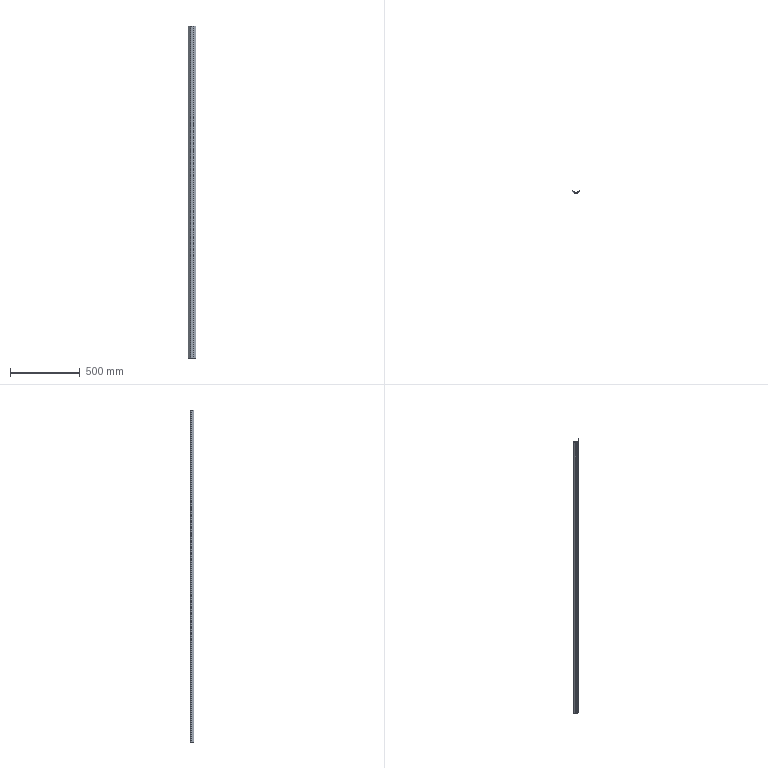Part | SolidWorks | features Extrusion 1 | 1 solid | 40 faces | box 56.572 x 22.358 x 2385 mm | volume 399812 mm3 | plane 37 | cylinder 3 | commonest cylinder face diameters 1 x2 0.5 x1
STEP:
#1=CARTESIAN_POINT('',(6.75,2.,-1192.5));
#2=VERTEX_POINT('',#1);
#3=CARTESIAN_POINT('',(6.75,5.,-1192.5));
#4=VERTEX_POINT('',#3);
#5=CARTESIAN_POINT('',(6.75,2.,-1192.5));
#6=DIRECTION('',(0.,1.,0.));
#7=VECTOR('',#6,1000.);
#8=LINE('',#5,#7);
#9=EDGE_CURVE('',#2,#4,#8,.T.);
#10=ORIENTED_EDGE('',*,*,#9,.T.);
#11=CARTESIAN_POINT('',(6.75,5.,1192.5));
#12=VERTEX_POINT('',#11);
#13=CARTESIAN_POINT('',(6.75,5.,1192.5));
#14=DIRECTION('',(0.,0.,-1.));
#15=VECTOR('',#14,1000.);
#16=LINE('',#13,#15);
#17=EDGE_CURVE('',#12,#4,#16,.T.);
#18=ORIENTED_EDGE('',*,*,#17,.F.);
#19=CARTESIAN_POINT('',(6.75,2.,1192.5));
#20=VERTEX_POINT('',#19);
#21=CARTESIAN_POINT('',(6.75,2.,1192.5));
#22=DIRECTION('',(0.,1.,0.));
#23=VECTOR('',#22,1000.);
#24=LINE('',#21,#23);
#25=EDGE_CURVE('',#20,#12,#24,.T.);
#26=ORIENTED_EDGE('',*,*,#25,.F.);
#27=CARTESIAN_POINT('',(6.75,2.,1192.5));
#28=DIRECTION('',(0.,0.,-1.));
#29=VECTOR('',#28,1000.);
#30=LINE('',#27,#29);
#31=EDGE_CURVE('',#20,#2,#30,.T.);
#32=ORIENTED_EDGE('',*,*,#31,.T.);
#33=EDGE_LOOP('',(#10,#18,#26,#32));
#34=FACE_OUTER_BOUND('',#33,.T.);
#35=CARTESIAN_POINT('',(6.75,2.,1192.5));
#36=DIRECTION('',(-1.,0.,0.));
#37=DIRECTION('',(0.,0.,1.));
#38=AXIS2_PLACEMENT_3D('',#35,#36,#37);
#39=PLANE('',#38);
#40=ADVANCED_FACE('',(#34),#39,.F.);
#41=CARTESIAN_POINT('',(5.25,5.,-1192.5));
#42=VERTEX_POINT('',#41);
#43=CARTESIAN_POINT('',(6.75,5.,-1192.5));
#44=DIRECTION('',(-1.,0.,0.));
#45=VECTOR('',#44,1000.);
#46=LINE('',#43,#45);
#47=EDGE_CURVE('',#4,#42,#46,.T.);
#48=ORIENTED_EDGE('',*,*,#47,.T.);
#49=CARTESIAN_POINT('',(5.25,5.,1192.5));
#50=VERTEX_POINT('',#49);
#51=CARTESIAN_POINT('',(5.25,5.,1192.5));
#52=DIRECTION('',(0.,0.,-1.));
#53=VECTOR('',#52,1000.);
#54=LINE('',#51,#53);
#55=EDGE_CURVE('',#50,#42,#54,.T.);
#56=ORIENTED_EDGE('',*,*,#55,.F.);
#57=CARTESIAN_POINT('',(6.75,5.,1192.5));
#58=DIRECTION('',(-1.,0.,0.));
#59=VECTOR('',#58,1000.);
#60=LINE('',#57,#59);
#61=EDGE_CURVE('',#12,#50,#60,.T.);
#62=ORIENTED_EDGE('',*,*,#61,.F.);
#63=ORIENTED_EDGE('',*,*,#17,.T.);
#64=EDGE_LOOP('',(#48,#56,#62,#63));
#65=FACE_OUTER_BOUND('',#64,.T.);
#66=CARTESIAN_POINT('',(6.75,5.,1192.5));
#67=DIRECTION('',(0.,-1.,0.));
#68=DIRECTION('',(1.,0.,0.));
#69=AXIS2_PLACEMENT_3D('',#66,#67,#68);
#70=PLANE('',#69);
#71=ADVANCED_FACE('',(#65),#70,.F.);
#72=CARTESIAN_POINT('',(5.25,2.,-1192.5));
#73=VERTEX_POINT('',#72);
#74=CARTESIAN_POINT('',(5.25,5.,-1192.5));
#75=DIRECTION('',(0.,-1.,0.));
#76=VECTOR('',#75,1000.);
#77=LINE('',#74,#76);
#78=EDGE_CURVE('',#42,#73,#77,.T.);
#79=ORIENTED_EDGE('',*,*,#78,.T.);
#80=CARTESIAN_POINT('',(5.25,2.,1192.5));
#81=VERTEX_POINT('',#80);
#82=CARTESIAN_POINT('',(5.25,2.,1192.5));
#83=DIRECTION('',(0.,0.,-1.));
#84=VECTOR('',#83,1000.);
#85=LINE('',#82,#84);
#86=EDGE_CURVE('',#81,#73,#85,.T.);
#87=ORIENTED_EDGE('',*,*,#86,.F.);
#88=CARTESIAN_POINT('',(5.25,5.,1192.5));
#89=DIRECTION('',(0.,-1.,0.));
#90=VECTOR('',#89,1000.);
#91=LINE('',#88,#90);
#92=EDGE_CURVE('',#50,#81,#91,.T.);
#93=ORIENTED_EDGE('',*,*,#92,.F.);
#94=ORIENTED_EDGE('',*,*,#55,.T.);
#95=EDGE_LOOP('',(#79,#87,#93,#94));
#96=FACE_OUTER_BOUND('',#95,.T.);
#97=CARTESIAN_POINT('',(5.25,5.,1192.5));
#98=DIRECTION('',(1.,0.,0.));
#99=DIRECTION('',(0.,0.,-1.));
#100=AXIS2_PLACEMENT_3D('',#97,#98,#99);
#101=PLANE('',#100);
#102=ADVANCED_FACE('',(#96),#101,.F.);
#103=CARTESIAN_POINT('',(0.25,2.,-1192.5));
#104=VERTEX_POINT('',#103);
#105=CARTESIAN_POINT('',(5.25,2.,-1192.5));
#106=DIRECTION('',(-1.,0.,0.));
#107=VECTOR('',#106,1000.);
#108=LINE('',#105,#107);
#109=EDGE_CURVE('',#73,#104,#108,.T.);
#110=ORIENTED_EDGE('',*,*,#109,.T.);
#111=CARTESIAN_POINT('',(0.25,2.,1192.5));
#112=VERTEX_POINT('',#111);
#113=CARTESIAN_POINT('',(0.25,2.,1192.5));
#114=DIRECTION('',(0.,0.,-1.));
#115=VECTOR('',#114,1000.);
#116=LINE('',#113,#115);
#117=EDGE_CURVE('',#112,#104,#116,.T.);
#118=ORIENTED_EDGE('',*,*,#117,.F.);
#119=CARTESIAN_POINT('',(5.25,2.,1192.5));
#120=DIRECTION('',(-1.,0.,0.));
#121=VECTOR('',#120,1000.);
#122=LINE('',#119,#121);
#123=EDGE_CURVE('',#81,#112,#122,.T.);
#124=ORIENTED_EDGE('',*,*,#123,.F.);
#125=ORIENTED_EDGE('',*,*,#86,.T.);
#126=EDGE_LOOP('',(#110,#118,#124,#125));
#127=FACE_OUTER_BOUND('',#126,.T.);
#128=CARTESIAN_POINT('',(5.25,2.,1192.5));
#129=DIRECTION('',(0.,-1.,0.));
#130=DIRECTION('',(0.,0.,-1.));
#131=AXIS2_PLACEMENT_3D('',#128,#129,#130);
#132=PLANE('',#131);
#133=ADVANCED_FACE('',(#127),#132,.F.);
#134=CARTESIAN_POINT('',(-0.25,2.,-1192.5));
#135=VERTEX_POINT('',#134);
#136=CARTESIAN_POINT('',(0.,2.,-1192.5));
#137=DIRECTION('',(0.,0.,-1.));
#138=DIRECTION('',(1.,0.,0.));
#139=AXIS2_PLACEMENT_3D('',#136,#137,#138);
#140=CIRCLE('',#139,0.25);
#141=EDGE_CURVE('',#104,#135,#140,.T.);
#142=ORIENTED_EDGE('',*,*,#141,.T.);
#143=CARTESIAN_POINT('',(-0.25,2.,1192.5));
#144=VERTEX_POINT('',#143);
#145=CARTESIAN_POINT('',(-0.25,2.,1192.5));
#146=DIRECTION('',(0.,0.,-1.));
#147=VECTOR('',#146,1000.);
#148=LINE('',#145,#147);
#149=EDGE_CURVE('',#144,#135,#148,.T.);
#150=ORIENTED_EDGE('',*,*,#149,.F.);
#151=CARTESIAN_POINT('',(0.,2.,1192.5));
#152=DIRECTION('',(0.,0.,-1.));
#153=DIRECTION('',(1.,0.,0.));
#154=AXIS2_PLACEMENT_3D('',#151,#152,#153);
#155=CIRCLE('',#154,0.25);
#156=EDGE_CURVE('',#112,#144,#155,.T.);
#157=ORIENTED_EDGE('',*,*,#156,.F.);
#158=ORIENTED_EDGE('',*,*,#117,.T.);
#159=EDGE_LOOP('',(#142,#150,#157,#158));
#160=FACE_OUTER_BOUND('',#159,.T.);
#161=CARTESIAN_POINT('',(0.,2.,1192.5));
#162=DIRECTION('',(0.,0.,-1.));
#163=DIRECTION('',(-1.,0.,0.));
#164=AXIS2_PLACEMENT_3D('',#161,#162,#163);
#165=CYLINDRICAL_SURFACE('',#164,0.25);
#166=ADVANCED_FACE('',(#160),#165,.F.);
#167=CARTESIAN_POINT('',(-5.25,2.,-1192.5));
#168=VERTEX_POINT('',#167);
#169=CARTESIAN_POINT('',(-0.25,2.,-1192.5));
#170=DIRECTION('',(-1.,0.,0.));
#171=VECTOR('',#170,1000.);
#172=LINE('',#169,#171);
#173=EDGE_CURVE('',#135,#168,#172,.T.);
#174=ORIENTED_EDGE('',*,*,#173,.T.);
#175=CARTESIAN_POINT('',(-5.25,2.,1192.5));
#176=VERTEX_POINT('',#175);
#177=CARTESIAN_POINT('',(-5.25,2.,1192.5));
#178=DIRECTION('',(0.,0.,-1.));
#179=VECTOR('',#178,1000.);
#180=LINE('',#177,#179);
#181=EDGE_CURVE('',#176,#168,#180,.T.);
#182=ORIENTED_EDGE('',*,*,#181,.F.);
#183=CARTESIAN_POINT('',(-0.25,2.,1192.5));
#184=DIRECTION('',(-1.,0.,0.));
#185=VECTOR('',#184,1000.);
#186=LINE('',#183,#185);
#187=EDGE_CURVE('',#144,#176,#186,.T.);
#188=ORIENTED_EDGE('',*,*,#187,.F.);
#189=ORIENTED_EDGE('',*,*,#149,.T.);
#190=EDGE_LOOP('',(#174,#182,#188,#189));
#191=FACE_OUTER_BOUND('',#190,.T.);
#192=CARTESIAN_POINT('',(-0.25,2.,1192.5));
#193=DIRECTION('',(0.,-1.,0.));
#194=DIRECTION('',(1.,0.,0.));
#195=AXIS2_PLACEMENT_3D('',#192,#193,#194);
#196=PLANE('',#195);
#197=ADVANCED_FACE('',(#191),#196,.F.);
#198=CARTESIAN_POINT('',(-5.25,5.,-1192.5));
#199=VERTEX_POINT('',#198);
#200=CARTESIAN_POINT('',(-5.25,2.,-1192.5));
#201=DIRECTION('',(0.,1.,0.));
#202=VECTOR('',#201,1000.);
#203=LINE('',#200,#202);
#204=EDGE_CURVE('',#168,#199,#203,.T.);
#205=ORIENTED_EDGE('',*,*,#204,.T.);
#206=CARTESIAN_POINT('',(-5.25,5.,1192.5));
#207=VERTEX_POINT('',#206);
#208=CARTESIAN_POINT('',(-5.25,5.,1192.5));
#209=DIRECTION('',(0.,0.,-1.));
#210=VECTOR('',#209,1000.);
#211=LINE('',#208,#210);
#212=EDGE_CURVE('',#207,#199,#211,.T.);
#213=ORIENTED_EDGE('',*,*,#212,.F.);
#214=CARTESIAN_POINT('',(-5.25,2.,1192.5));
#215=DIRECTION('',(0.,1.,0.));
#216=VECTOR('',#215,1000.);
#217=LINE('',#214,#216);
#218=EDGE_CURVE('',#176,#207,#217,.T.);
#219=ORIENTED_EDGE('',*,*,#218,.F.);
#220=ORIENTED_EDGE('',*,*,#181,.T.);
#221=EDGE_LOOP('',(#205,#213,#219,#220));
#222=FACE_OUTER_BOUND('',#221,.T.);
#223=CARTESIAN_POINT('',(-5.25,2.,1192.5));
#224=DIRECTION('',(-1.,0.,0.));
#225=DIRECTION('',(0.,0.,1.));
#226=AXIS2_PLACEMENT_3D('',#223,#224,#225);
#227=PLANE('',#226);
#228=ADVANCED_FACE('',(#222),#227,.F.);
#229=CARTESIAN_POINT('',(-6.75,5.,-1192.5));
#230=VERTEX_POINT('',#229);
#231=CARTESIAN_POINT('',(-5.25,5.,-1192.5));
#232=DIRECTION('',(-1.,0.,0.));
#233=VECTOR('',#232,1000.);
#234=LINE('',#231,#233);
#235=EDGE_CURVE('',#199,#230,#234,.T.);
#236=ORIENTED_EDGE('',*,*,#235,.T.);
#237=CARTESIAN_POINT('',(-6.75,5.,1192.5));
#238=VERTEX_POINT('',#237);
#239=CARTESIAN_POINT('',(-6.75,5.,1192.5));
#240=DIRECTION('',(0.,0.,-1.));
#241=VECTOR('',#240,1000.);
#242=LINE('',#239,#241);
#243=EDGE_CURVE('',#238,#230,#242,.T.);
#244=ORIENTED_EDGE('',*,*,#243,.F.);
#245=CARTESIAN_POINT('',(-5.25,5.,1192.5));
#246=DIRECTION('',(-1.,0.,0.));
#247=VECTOR('',#246,1000.);
#248=LINE('',#245,#247);
#249=EDGE_CURVE('',#207,#238,#248,.T.);
#250=ORIENTED_EDGE('',*,*,#249,.F.);
#251=ORIENTED_EDGE('',*,*,#212,.T.);
#252=EDGE_LOOP('',(#236,#244,#250,#251));
#253=FACE_OUTER_BOUND('',#252,.T.);
#254=CARTESIAN_POINT('',(-5.25,5.,1192.5));
#255=DIRECTION('',(0.,-1.,0.));
#256=DIRECTION('',(1.,0.,0.));
#257=AXIS2_PLACEMENT_3D('',#254,#255,#256);
#258=PLANE('',#257);
#259=ADVANCED_FACE('',(#253),#258,.F.);
#260=CARTESIAN_POINT('',(-6.75,2.,-1192.5));
#261=VERTEX_POINT('',#260);
#262=CARTESIAN_POINT('',(-6.75,5.,-1192.5));
#263=DIRECTION('',(0.,-1.,0.));
#264=VECTOR('',#263,1000.);
#265=LINE('',#262,#264);
#266=EDGE_CURVE('',#230,#261,#265,.T.);
#267=ORIENTED_EDGE('',*,*,#266,.T.);
#268=CARTESIAN_POINT('',(-6.75,2.,1192.5));
#269=VERTEX_POINT('',#268);
#270=CARTESIAN_POINT('',(-6.75,2.,1192.5));
#271=DIRECTION('',(0.,0.,-1.));
#272=VECTOR('',#271,1000.);
#273=LINE('',#270,#272);
#274=EDGE_CURVE('',#269,#261,#273,.T.);
#275=ORIENTED_EDGE('',*,*,#274,.F.);
#276=CARTESIAN_POINT('',(-6.75,5.,1192.5));
#277=DIRECTION('',(0.,-1.,0.));
#278=VECTOR('',#277,1000.);
#279=LINE('',#276,#278);
#280=EDGE_CURVE('',#238,#269,#279,.T.);
#281=ORIENTED_EDGE('',*,*,#280,.F.);
#282=ORIENTED_EDGE('',*,*,#243,.T.);
#283=EDGE_LOOP('',(#267,#275,#281,#282));
#284=FACE_OUTER_BOUND('',#283,.T.);
#285=CARTESIAN_POINT('',(-6.75,5.,1192.5));
#286=DIRECTION('',(1.,0.,0.));
#287=DIRECTION('',(0.,0.,-1.));
#288=AXIS2_PLACEMENT_3D('',#285,#286,#287);
#289=PLANE('',#288);
#290=ADVANCED_FACE('',(#284),#289,.F.);
#291=CARTESIAN_POINT('',(-8.635,2.,-1192.5));
#292=VERTEX_POINT('',#291);
#293=CARTESIAN_POINT('',(-6.75,2.,-1192.5));
#294=DIRECTION('',(-1.,0.,0.));
#295=VECTOR('',#294,1000.);
#296=LINE('',#293,#295);
#297=EDGE_CURVE('',#261,#292,#296,.T.);
#298=ORIENTED_EDGE('',*,*,#297,.T.);
#299=CARTESIAN_POINT('',(-8.635,2.,1192.5));
#300=VERTEX_POINT('',#299);
#301=CARTESIAN_POINT('',(-8.635,2.,1192.5));
#302=DIRECTION('',(0.,0.,-1.));
#303=VECTOR('',#302,1000.);
#304=LINE('',#301,#303);
#305=EDGE_CURVE('',#300,#292,#304,.T.);
#306=ORIENTED_EDGE('',*,*,#305,.F.);
#307=CARTESIAN_POINT('',(-6.75,2.,1192.5));
#308=DIRECTION('',(-1.,0.,0.));
#309=VECTOR('',#308,1000.);
#310=LINE('',#307,#309);
#311=EDGE_CURVE('',#269,#300,#310,.T.);
#312=ORIENTED_EDGE('',*,*,#311,.F.);
#313=ORIENTED_EDGE('',*,*,#274,.T.);
#314=EDGE_LOOP('',(#298,#306,#312,#313));
#315=FACE_OUTER_BOUND('',#314,.T.);
#316=CARTESIAN_POINT('',(-6.75,2.,1192.5));
#317=DIRECTION('',(0.,-1.,0.));
#318=DIRECTION('',(1.,0.,0.));
#319=AXIS2_PLACEMENT_3D('',#316,#317,#318);
#320=PLANE('',#319);
#321=ADVANCED_FACE('',(#315),#320,.F.);
#322=CARTESIAN_POINT('',(-11.75,5.119,-1192.5));
#323=VERTEX_POINT('',#322);
#324=CARTESIAN_POINT('',(-8.635,2.,-1192.5));
#325=DIRECTION('',(-0.7067,0.7076,0.));
#326=VECTOR('',#325,1000.);
#327=LINE('',#324,#326);
#328=EDGE_CURVE('',#292,#323,#327,.T.);
#329=ORIENTED_EDGE('',*,*,#328,.T.);
#330=CARTESIAN_POINT('',(-11.75,5.119,1192.5));
#331=VERTEX_POINT('',#330);
#332=CARTESIAN_POINT('',(-11.75,5.119,1192.5));
#333=DIRECTION('',(0.,0.,-1.));
#334=VECTOR('',#333,1000.);
#335=LINE('',#332,#334);
#336=EDGE_CURVE('',#331,#323,#335,.T.);
#337=ORIENTED_EDGE('',*,*,#336,.F.);
#338=CARTESIAN_POINT('',(-8.635,2.,1192.5));
#339=DIRECTION('',(-0.7067,0.7076,0.));
#340=VECTOR('',#339,1000.);
#341=LINE('',#338,#340);
#342=EDGE_CURVE('',#300,#331,#341,.T.);
#343=ORIENTED_EDGE('',*,*,#342,.F.);
#344=ORIENTED_EDGE('',*,*,#305,.T.);
#345=EDGE_LOOP('',(#329,#337,#343,#344));
#346=FACE_OUTER_BOUND('',#345,.T.);
#347=CARTESIAN_POINT('',(-8.635,2.,1192.5));
#348=DIRECTION('',(-0.7076,-0.7067,0.));
#349=DIRECTION('',(0.7067,-0.7076,0.));
#350=AXIS2_PLACEMENT_3D('',#347,#348,#349);
#351=PLANE('',#350);
#352=ADVANCED_FACE('',(#346),#351,.F.);
#353=CARTESIAN_POINT('',(-11.75,8.887,-1192.5));
#354=VERTEX_POINT('',#353);
#355=CARTESIAN_POINT('',(-11.75,5.119,-1192.5));
#356=DIRECTION('',(0.,1.,0.));
#357=VECTOR('',#356,1000.);
#358=LINE('',#355,#357);
#359=EDGE_CURVE('',#323,#354,#358,.T.);
#360=ORIENTED_EDGE('',*,*,#359,.T.);
#361=CARTESIAN_POINT('',(-11.75,8.887,1192.5));
#362=VERTEX_POINT('',#361);
#363=CARTESIAN_POINT('',(-11.75,8.887,1192.5));
#364=DIRECTION('',(0.,0.,-1.));
#365=VECTOR('',#364,1000.);
#366=LINE('',#363,#365);
#367=EDGE_CURVE('',#362,#354,#366,.T.);
#368=ORIENTED_EDGE('',*,*,#367,.F.);
#369=CARTESIAN_POINT('',(-11.75,5.119,1192.5));
#370=DIRECTION('',(0.,1.,0.));
#371=VECTOR('',#370,1000.);
#372=LINE('',#369,#371);
#373=EDGE_CURVE('',#331,#362,#372,.T.);
#374=ORIENTED_EDGE('',*,*,#373,.F.);
#375=ORIENTED_EDGE('',*,*,#336,.T.);
#376=EDGE_LOOP('',(#360,#368,#374,#375));
#377=FACE_OUTER_BOUND('',#376,.T.);
#378=CARTESIAN_POINT('',(-11.75,5.119,1192.5));
#379=DIRECTION('',(-1.,0.,0.));
#380=DIRECTION('',(0.,0.,1.));
#381=AXIS2_PLACEMENT_3D('',#378,#379,#380);
#382=PLANE('',#381);
#383=ADVANCED_FACE('',(#377),#382,.F.);
#384=CARTESIAN_POINT('',(-12.25,9.387,-1192.5));
#385=VERTEX_POINT('',#384);
#386=CARTESIAN_POINT('',(-11.75,8.887,-1192.5));
#387=DIRECTION('',(-0.7071,0.7071,0.));
#388=VECTOR('',#387,1000.);
#389=LINE('',#386,#388);
#390=EDGE_CURVE('',#354,#385,#389,.T.);
#391=ORIENTED_EDGE('',*,*,#390,.T.);
#392=CARTESIAN_POINT('',(-12.25,9.387,1192.5));
#393=VERTEX_POINT('',#392);
#394=CARTESIAN_POINT('',(-12.25,9.387,1192.5));
#395=DIRECTION('',(0.,0.,-1.));
#396=VECTOR('',#395,1000.);
#397=LINE('',#394,#396);
#398=EDGE_CURVE('',#393,#385,#397,.T.);
#399=ORIENTED_EDGE('',*,*,#398,.F.);
#400=CARTESIAN_POINT('',(-11.75,8.887,1192.5));
#401=DIRECTION('',(-0.7071,0.7071,0.));
#402=VECTOR('',#401,1000.);
#403=LINE('',#400,#402);
#404=EDGE_CURVE('',#362,#393,#403,.T.);
#405=ORIENTED_EDGE('',*,*,#404,.F.);
#406=ORIENTED_EDGE('',*,*,#367,.T.);
#407=EDGE_LOOP('',(#391,#399,#405,#406));
#408=FACE_OUTER_BOUND('',#407,.T.);
#409=CARTESIAN_POINT('',(-11.75,8.887,1192.5));
#410=DIRECTION('',(-0.7071,-0.7071,0.));
#411=DIRECTION('',(0.7071,-0.7071,0.));
#412=AXIS2_PLACEMENT_3D('',#409,#410,#411);
#413=PLANE('',#412);
#414=ADVANCED_FACE('',(#408),#413,.F.);
#415=CARTESIAN_POINT('',(-12.75,9.387,-1192.5));
#416=VERTEX_POINT('',#415);
#417=CARTESIAN_POINT('',(-12.25,9.387,-1192.5));
#418=DIRECTION('',(-1.,0.,0.));
#419=VECTOR('',#418,1000.);
#420=LINE('',#417,#419);
#421=EDGE_CURVE('',#385,#416,#420,.T.);
#422=ORIENTED_EDGE('',*,*,#421,.T.);
#423=CARTESIAN_POINT('',(-12.75,9.387,1192.5));
#424=VERTEX_POINT('',#423);
#425=CARTESIAN_POINT('',(-12.75,9.387,1192.5));
#426=DIRECTION('',(0.,0.,-1.));
#427=VECTOR('',#426,1000.);
#428=LINE('',#425,#427);
#429=EDGE_CURVE('',#424,#416,#428,.T.);
#430=ORIENTED_EDGE('',*,*,#429,.F.);
#431=CARTESIAN_POINT('',(-12.25,9.387,1192.5));
#432=DIRECTION('',(-1.,0.,0.));
#433=VECTOR('',#432,1000.);
#434=LINE('',#431,#433);
#435=EDGE_CURVE('',#393,#424,#434,.T.);
#436=ORIENTED_EDGE('',*,*,#435,.F.);
#437=ORIENTED_EDGE('',*,*,#398,.T.);
#438=EDGE_LOOP('',(#422,#430,#436,#437));
#439=FACE_OUTER_BOUND('',#438,.T.);
#440=CARTESIAN_POINT('',(-12.25,9.387,1192.5));
#441=DIRECTION('',(0.,-1.,0.));
#442=DIRECTION('',(0.,0.,-1.));
#443=AXIS2_PLACEMENT_3D('',#440,#441,#442);
#444=PLANE('',#443);
#445=ADVANCED_FACE('',(#439),#444,.F.);
#446=CARTESIAN_POINT('',(-12.75,7.328,-1192.5));
#447=VERTEX_POINT('',#446);
#448=CARTESIAN_POINT('',(-12.75,9.387,-1192.5));
#449=DIRECTION('',(0.,-1.,0.));
#450=VECTOR('',#449,1000.);
#451=LINE('',#448,#450);
#452=EDGE_CURVE('',#416,#447,#451,.T.);
#453=ORIENTED_EDGE('',*,*,#452,.T.);
#454=CARTESIAN_POINT('',(-12.75,7.328,1192.5));
#455=VERTEX_POINT('',#454);
#456=CARTESIAN_POINT('',(-12.75,7.328,1192.5));
#457=DIRECTION('',(0.,0.,-1.));
#458=VECTOR('',#457,1000.);
#459=LINE('',#456,#458);
#460=EDGE_CURVE('',#455,#447,#459,.T.);
#461=ORIENTED_EDGE('',*,*,#460,.F.);
#462=CARTESIAN_POINT('',(-12.75,9.387,1192.5));
#463=DIRECTION('',(0.,-1.,0.));
#464=VECTOR('',#463,1000.);
#465=LINE('',#462,#464);
#466=EDGE_CURVE('',#424,#455,#465,.T.);
#467=ORIENTED_EDGE('',*,*,#466,.F.);
#468=ORIENTED_EDGE('',*,*,#429,.T.);
#469=EDGE_LOOP('',(#453,#461,#467,#468));
#470=FACE_OUTER_BOUND('',#469,.T.);
#471=CARTESIAN_POINT('',(-12.75,9.387,1192.5));
#472=DIRECTION('',(1.,0.,0.));
#473=DIRECTION('',(0.,0.,-1.));
#474=AXIS2_PLACEMENT_3D('',#471,#472,#473);
#475=PLANE('',#474);
#476=ADVANCED_FACE('',(#470),#475,.F.);
#477=CARTESIAN_POINT('',(-13.604,6.975,-1192.5));
#478=VERTEX_POINT('',#477);
#479=CARTESIAN_POINT('',(-13.25,7.328,-1192.5));
#480=DIRECTION('',(0.,0.,-1.));
#481=DIRECTION('',(1.,0.,0.));
#482=AXIS2_PLACEMENT_3D('',#479,#480,#481);
#483=CIRCLE('',#482,0.5);
#484=EDGE_CURVE('',#447,#478,#483,.T.);
#485=ORIENTED_EDGE('',*,*,#484,.T.);
#486=CARTESIAN_POINT('',(-13.604,6.975,1192.5));
#487=VERTEX_POINT('',#486);
#488=CARTESIAN_POINT('',(-13.604,6.975,1192.5));
#489=DIRECTION('',(0.,0.,-1.));
#490=VECTOR('',#489,1000.);
#491=LINE('',#488,#490);
#492=EDGE_CURVE('',#487,#478,#491,.T.);
#493=ORIENTED_EDGE('',*,*,#492,.F.);
#494=CARTESIAN_POINT('',(-13.25,7.328,1192.5));
#495=DIRECTION('',(0.,0.,-1.));
#496=DIRECTION('',(1.,0.,0.));
#497=AXIS2_PLACEMENT_3D('',#494,#495,#496);
#498=CIRCLE('',#497,0.5);
#499=EDGE_CURVE('',#455,#487,#498,.T.);
#500=ORIENTED_EDGE('',*,*,#499,.F.);
#501=ORIENTED_EDGE('',*,*,#460,.T.);
#502=EDGE_LOOP('',(#485,#493,#500,#501));
#503=FACE_OUTER_BOUND('',#502,.T.);
#504=CARTESIAN_POINT('',(-13.25,7.328,1192.5));
#505=DIRECTION('',(0.,0.,-1.));
#506=DIRECTION('',(-1.,0.,0.));
#507=AXIS2_PLACEMENT_3D('',#504,#505,#506);
#508=CYLINDRICAL_SURFACE('',#507,0.5);
#509=ADVANCED_FACE('',(#503),#508,.F.);
#510=CARTESIAN_POINT('',(-23.891,17.282,-1192.5));
#511=VERTEX_POINT('',#510);
#512=CARTESIAN_POINT('',(-13.604,6.975,-1192.5));
#513=DIRECTION('',(-0.7064,0.7078,0.));
#514=VECTOR('',#513,1000.);
#515=LINE('',#512,#514);
#516=EDGE_CURVE('',#478,#511,#515,.T.);
#517=ORIENTED_EDGE('',*,*,#516,.T.);
#518=CARTESIAN_POINT('',(-23.891,17.282,1192.5));
#519=VERTEX_POINT('',#518);
#520=CARTESIAN_POINT('',(-23.891,17.282,1192.5));
#521=DIRECTION('',(0.,0.,-1.));
#522=VECTOR('',#521,1000.);
#523=LINE('',#520,#522);
#524=EDGE_CURVE('',#519,#511,#523,.T.);
#525=ORIENTED_EDGE('',*,*,#524,.F.);
#526=CARTESIAN_POINT('',(-13.604,6.975,1192.5));
#527=DIRECTION('',(-0.7064,0.7078,0.));
#528=VECTOR('',#527,1000.);
#529=LINE('',#526,#528);
#530=EDGE_CURVE('',#487,#519,#529,.T.);
#531=ORIENTED_EDGE('',*,*,#530,.F.);
#532=ORIENTED_EDGE('',*,*,#492,.T.);
#533=EDGE_LOOP('',(#517,#525,#531,#532));
#534=FACE_OUTER_BOUND('',#533,.T.);
#535=CARTESIAN_POINT('',(-13.604,6.975,1192.5));
#536=DIRECTION('',(-0.7078,-0.7064,0.));
#537=DIRECTION('',(0.7064,-0.7078,0.));
#538=AXIS2_PLACEMENT_3D('',#535,#536,#537);
#539=PLANE('',#538);
#540=ADVANCED_FACE('',(#534),#539,.F.);
#541=CARTESIAN_POINT('',(-23.891,19.376,-1192.5));
#542=VERTEX_POINT('',#541);
#543=CARTESIAN_POINT('',(-23.891,17.282,-1192.5));
#544=DIRECTION('',(0.,1.,0.));
#545=VECTOR('',#544,1000.);
#546=LINE('',#543,#545);
#547=EDGE_CURVE('',#511,#542,#546,.T.);
#548=ORIENTED_EDGE('',*,*,#547,.T.);
#549=CARTESIAN_POINT('',(-23.891,19.376,1192.5));
#550=VERTEX_POINT('',#549);
#551=CARTESIAN_POINT('',(-23.891,19.376,1192.5));
#552=DIRECTION('',(0.,0.,-1.));
#553=VECTOR('',#552,1000.);
#554=LINE('',#551,#553);
#555=EDGE_CURVE('',#550,#542,#554,.T.);
#556=ORIENTED_EDGE('',*,*,#555,.F.);
#557=CARTESIAN_POINT('',(-23.891,17.282,1192.5));
#558=DIRECTION('',(0.,1.,0.));
#559=VECTOR('',#558,1000.);
#560=LINE('',#557,#559);
#561=EDGE_CURVE('',#519,#550,#560,.T.);
#562=ORIENTED_EDGE('',*,*,#561,.F.);
#563=ORIENTED_EDGE('',*,*,#524,.T.);
#564=EDGE_LOOP('',(#548,#556,#562,#563));
#565=FACE_OUTER_BOUND('',#564,.T.);
#566=CARTESIAN_POINT('',(-23.891,17.282,1192.5));
#567=DIRECTION('',(-1.,0.,0.));
#568=DIRECTION('',(0.,0.,1.));
#569=AXIS2_PLACEMENT_3D('',#566,#567,#568);
#570=PLANE('',#569);
#571=ADVANCED_FACE('',(#565),#570,.F.);
#572=CARTESIAN_POINT('',(-26.873,22.358,-1192.5));
#573=VERTEX_POINT('',#572);
#574=CARTESIAN_POINT('',(-23.891,19.376,-1192.5));
#575=DIRECTION('',(-0.7071,0.7071,0.));
#576=VECTOR('',#575,1000.);
#577=LINE('',#574,#576);
#578=EDGE_CURVE('',#542,#573,#577,.T.);
#579=ORIENTED_EDGE('',*,*,#578,.T.);
#580=CARTESIAN_POINT('',(-26.873,22.358,1192.5));
#581=VERTEX_POINT('',#580);
#582=CARTESIAN_POINT('',(-26.873,22.358,1192.5));
#583=DIRECTION('',(0.,0.,-1.));
#584=VECTOR('',#583,1000.);
#585=LINE('',#582,#584);
#586=EDGE_CURVE('',#581,#573,#585,.T.);
#587=ORIENTED_EDGE('',*,*,#586,.F.);
#588=CARTESIAN_POINT('',(-23.891,19.376,1192.5));
#589=DIRECTION('',(-0.7071,0.7071,0.));
#590=VECTOR('',#589,1000.);
#591=LINE('',#588,#590);
#592=EDGE_CURVE('',#550,#581,#591,.T.);
#593=ORIENTED_EDGE('',*,*,#592,.F.);
#594=ORIENTED_EDGE('',*,*,#555,.T.);
#595=EDGE_LOOP('',(#579,#587,#593,#594));
#596=FACE_OUTER_BOUND('',#595,.T.);
#597=CARTESIAN_POINT('',(-23.891,19.376,1192.5));
#598=DIRECTION('',(-0.7071,-0.7071,0.));
#599=DIRECTION('',(0.7071,-0.7071,0.));
#600=AXIS2_PLACEMENT_3D('',#597,#598,#599);
#601=PLANE('',#600);
#602=ADVANCED_FACE('',(#596),#601,.F.);
#603=CARTESIAN_POINT('',(-27.58,22.358,-1192.5));
#604=VERTEX_POINT('',#603);
#605=CARTESIAN_POINT('',(-26.873,22.358,-1192.5));
#606=DIRECTION('',(-1.,0.,0.));
#607=VECTOR('',#606,1000.);
#608=LINE('',#605,#607);
#609=EDGE_CURVE('',#573,#604,#608,.T.);
#610=ORIENTED_EDGE('',*,*,#609,.T.);
#611=CARTESIAN_POINT('',(-27.58,22.358,1192.5));
#612=VERTEX_POINT('',#611);
#613=CARTESIAN_POINT('',(-27.58,22.358,1192.5));
#614=DIRECTION('',(0.,0.,-1.));
#615=VECTOR('',#614,1000.);
#616=LINE('',#613,#615);
#617=EDGE_CURVE('',#612,#604,#616,.T.);
#618=ORIENTED_EDGE('',*,*,#617,.F.);
#619=CARTESIAN_POINT('',(-26.873,22.358,1192.5));
#620=DIRECTION('',(-1.,0.,0.));
#621=VECTOR('',#620,1000.);
#622=LINE('',#619,#621);
#623=EDGE_CURVE('',#581,#612,#622,.T.);
#624=ORIENTED_EDGE('',*,*,#623,.F.);
#625=ORIENTED_EDGE('',*,*,#586,.T.);
#626=EDGE_LOOP('',(#610,#618,#624,#625));
#627=FACE_OUTER_BOUND('',#626,.T.);
#628=CARTESIAN_POINT('',(-26.873,22.358,1192.5));
#629=DIRECTION('',(0.,-1.,0.));
#630=DIRECTION('',(0.,0.,-1.));
#631=AXIS2_PLACEMENT_3D('',#628,#629,#630);
#632=PLANE('',#631);
#633=ADVANCED_FACE('',(#627),#632,.F.);
#634=CARTESIAN_POINT('',(-28.284,21.654,-1192.5));
#635=VERTEX_POINT('',#634);
#636=CARTESIAN_POINT('',(-27.58,22.358,-1192.5));
#637=DIRECTION('',(-0.7071,-0.7071,0.));
#638=VECTOR('',#637,1000.);
#639=LINE('',#636,#638);
#640=EDGE_CURVE('',#604,#635,#639,.T.);
#641=ORIENTED_EDGE('',*,*,#640,.T.);
#642=CARTESIAN_POINT('',(-28.284,21.654,1192.5));
#643=VERTEX_POINT('',#642);
#644=CARTESIAN_POINT('',(-28.284,21.654,1192.5));
#645=DIRECTION('',(0.,0.,-1.));
#646=VECTOR('',#645,1000.);
#647=LINE('',#644,#646);
#648=EDGE_CURVE('',#643,#635,#647,.T.);
#649=ORIENTED_EDGE('',*,*,#648,.F.);
#650=CARTESIAN_POINT('',(-27.58,22.358,1192.5));
#651=DIRECTION('',(-0.7071,-0.7071,0.));
#652=VECTOR('',#651,1000.);
#653=LINE('',#650,#652);
#654=EDGE_CURVE('',#612,#643,#653,.T.);
#655=ORIENTED_EDGE('',*,*,#654,.F.);
#656=ORIENTED_EDGE('',*,*,#617,.T.);
#657=EDGE_LOOP('',(#641,#649,#655,#656));
#658=FACE_OUTER_BOUND('',#657,.T.);
#659=CARTESIAN_POINT('',(-27.58,22.358,1192.5));
#660=DIRECTION('',(0.7071,-0.7071,0.));
#661=DIRECTION('',(0.7071,0.7071,0.));
#662=AXIS2_PLACEMENT_3D('',#659,#660,#661);
#663=PLANE('',#662);
#664=ADVANCED_FACE('',(#658),#663,.F.);
#665=CARTESIAN_POINT('',(-28.284,19.103,-1192.5));
#666=VERTEX_POINT('',#665);
#667=CARTESIAN_POINT('',(-28.284,21.654,-1192.5));
#668=DIRECTION('',(0.,-1.,0.));
#669=VECTOR('',#668,1000.);
#670=LINE('',#667,#669);
#671=EDGE_CURVE('',#635,#666,#670,.T.);
#672=ORIENTED_EDGE('',*,*,#671,.T.);
#673=CARTESIAN_POINT('',(-28.284,19.103,1192.5));
#674=VERTEX_POINT('',#673);
#675=CARTESIAN_POINT('',(-28.284,19.103,1192.5));
#676=DIRECTION('',(0.,0.,-1.));
#677=VECTOR('',#676,1000.);
#678=LINE('',#675,#677);
#679=EDGE_CURVE('',#674,#666,#678,.T.);
#680=ORIENTED_EDGE('',*,*,#679,.F.);
#681=CARTESIAN_POINT('',(-28.284,21.654,1192.5));
#682=DIRECTION('',(0.,-1.,0.));
#683=VECTOR('',#682,1000.);
#684=LINE('',#681,#683);
#685=EDGE_CURVE('',#643,#674,#684,.T.);
#686=ORIENTED_EDGE('',*,*,#685,.F.);
#687=ORIENTED_EDGE('',*,*,#648,.T.);
#688=EDGE_LOOP('',(#672,#680,#686,#687));
#689=FACE_OUTER_BOUND('',#688,.T.);
#690=CARTESIAN_POINT('',(-28.284,21.654,1192.5));
#691=DIRECTION('',(1.,0.,0.));
#692=DIRECTION('',(0.,0.,-1.));
#693=AXIS2_PLACEMENT_3D('',#690,#691,#692);
#694=PLANE('',#693);
#695=ADVANCED_FACE('',(#689),#694,.F.);
#696=CARTESIAN_POINT('',(-9.182,0.,-1192.5));
#697=VERTEX_POINT('',#696);
#698=CARTESIAN_POINT('',(-28.284,19.103,-1192.5));
#699=DIRECTION('',(0.7071,-0.7071,0.));
#700=VECTOR('',#699,1000.);
#701=LINE('',#698,#700);
#702=EDGE_CURVE('',#666,#697,#701,.T.);
#703=ORIENTED_EDGE('',*,*,#702,.T.);
#704=CARTESIAN_POINT('',(-9.182,0.,1192.5));
#705=VERTEX_POINT('',#704);
#706=CARTESIAN_POINT('',(-9.182,0.,1192.5));
#707=DIRECTION('',(0.,0.,-1.));
#708=VECTOR('',#707,1000.);
#709=LINE('',#706,#708);
#710=EDGE_CURVE('',#705,#697,#709,.T.);
#711=ORIENTED_EDGE('',*,*,#710,.F.);
#712=CARTESIAN_POINT('',(-28.284,19.103,1192.5));
#713=DIRECTION('',(0.7071,-0.7071,0.));
#714=VECTOR('',#713,1000.);
#715=LINE('',#712,#714);
#716=EDGE_CURVE('',#674,#705,#715,.T.);
#717=ORIENTED_EDGE('',*,*,#716,.F.);
#718=ORIENTED_EDGE('',*,*,#679,.T.);
#719=EDGE_LOOP('',(#703,#711,#717,#718));
#720=FACE_OUTER_BOUND('',#719,.T.);
#721=CARTESIAN_POINT('',(-28.284,19.103,1192.5));
#722=DIRECTION('',(0.7071,0.7071,0.));
#723=DIRECTION('',(-0.7071,0.7071,0.));
#724=AXIS2_PLACEMENT_3D('',#721,#722,#723);
#725=PLANE('',#724);
#726=ADVANCED_FACE('',(#720),#725,.F.);
#727=CARTESIAN_POINT('',(9.182,0.,-1192.5));
#728=VERTEX_POINT('',#727);
#729=CARTESIAN_POINT('',(-9.182,0.,-1192.5));
#730=DIRECTION('',(1.,0.,0.));
#731=VECTOR('',#730,1000.);
#732=LINE('',#729,#731);
#733=EDGE_CURVE('',#697,#728,#732,.T.);
#734=ORIENTED_EDGE('',*,*,#733,.T.);
#735=CARTESIAN_POINT('',(9.182,0.,1192.5));
#736=VERTEX_POINT('',#735);
#737=CARTESIAN_POINT('',(9.182,0.,1192.5));
#738=DIRECTION('',(0.,0.,-1.));
#739=VECTOR('',#738,1000.);
#740=LINE('',#737,#739);
#741=EDGE_CURVE('',#736,#728,#740,.T.);
#742=ORIENTED_EDGE('',*,*,#741,.F.);
#743=CARTESIAN_POINT('',(-9.182,0.,1192.5));
#744=DIRECTION('',(1.,0.,0.));
#745=VECTOR('',#744,1000.);
#746=LINE('',#743,#745);
#747=EDGE_CURVE('',#705,#736,#746,.T.);
#748=ORIENTED_EDGE('',*,*,#747,.F.);
#749=ORIENTED_EDGE('',*,*,#710,.T.);
#750=EDGE_LOOP('',(#734,#742,#748,#749));
#751=FACE_OUTER_BOUND('',#750,.T.);
#752=CARTESIAN_POINT('',(-9.182,0.,1192.5));
#753=DIRECTION('',(0.,1.,0.));
#754=DIRECTION('',(-1.,0.,0.));
#755=AXIS2_PLACEMENT_3D('',#752,#753,#754);
#756=PLANE('',#755);
#757=ADVANCED_FACE('',(#751),#756,.F.);
#758=CARTESIAN_POINT('',(28.287,19.106,-1192.5));
#759=VERTEX_POINT('',#758);
#760=CARTESIAN_POINT('',(9.182,0.,-1192.5));
#761=DIRECTION('',(0.7071,0.7071,0.));
#762=VECTOR('',#761,1000.);
#763=LINE('',#760,#762);
#764=EDGE_CURVE('',#728,#759,#763,.T.);
#765=ORIENTED_EDGE('',*,*,#764,.T.);
#766=CARTESIAN_POINT('',(28.287,19.106,1192.5));
#767=VERTEX_POINT('',#766);
#768=CARTESIAN_POINT('',(28.287,19.106,1192.5));
#769=DIRECTION('',(0.,0.,-1.));
#770=VECTOR('',#769,1000.);
#771=LINE('',#768,#770);
#772=EDGE_CURVE('',#767,#759,#771,.T.);
#773=ORIENTED_EDGE('',*,*,#772,.F.);
#774=CARTESIAN_POINT('',(9.182,0.,1192.5));
#775=DIRECTION('',(0.7071,0.7071,0.));
#776=VECTOR('',#775,1000.);
#777=LINE('',#774,#776);
#778=EDGE_CURVE('',#736,#767,#777,.T.);
#779=ORIENTED_EDGE('',*,*,#778,.F.);
#780=ORIENTED_EDGE('',*,*,#741,.T.);
#781=EDGE_LOOP('',(#765,#773,#779,#780));
#782=FACE_OUTER_BOUND('',#781,.T.);
#783=CARTESIAN_POINT('',(9.182,0.,1192.5));
#784=DIRECTION('',(-0.7071,0.7071,0.));
#785=DIRECTION('',(-0.7071,-0.7071,0.));
#786=AXIS2_PLACEMENT_3D('',#783,#784,#785);
#787=PLANE('',#786);
#788=ADVANCED_FACE('',(#782),#787,.F.);
#789=CARTESIAN_POINT('',(28.287,21.651,-1192.5));
#790=VERTEX_POINT('',#789);
#791=CARTESIAN_POINT('',(28.287,19.106,-1192.5));
#792=DIRECTION('',(0.,1.,0.));
#793=VECTOR('',#792,1000.);
#794=LINE('',#791,#793);
#795=EDGE_CURVE('',#759,#790,#794,.T.);
#796=ORIENTED_EDGE('',*,*,#795,.T.);
#797=CARTESIAN_POINT('',(28.287,21.651,1192.5));
#798=VERTEX_POINT('',#797);
#799=CARTESIAN_POINT('',(28.287,21.651,1192.5));
#800=DIRECTION('',(0.,0.,-1.));
#801=VECTOR('',#800,1000.);
#802=LINE('',#799,#801);
#803=EDGE_CURVE('',#798,#790,#802,.T.);
#804=ORIENTED_EDGE('',*,*,#803,.F.);
#805=CARTESIAN_POINT('',(28.287,19.106,1192.5));
#806=DIRECTION('',(0.,1.,0.));
#807=VECTOR('',#806,1000.);
#808=LINE('',#805,#807);
#809=EDGE_CURVE('',#767,#798,#808,.T.);
#810=ORIENTED_EDGE('',*,*,#809,.F.);
#811=ORIENTED_EDGE('',*,*,#772,.T.);
#812=EDGE_LOOP('',(#796,#804,#810,#811));
#813=FACE_OUTER_BOUND('',#812,.T.);
#814=CARTESIAN_POINT('',(28.287,19.106,1192.5));
#815=DIRECTION('',(-1.,0.,0.));
#816=DIRECTION('',(0.,-1.,0.));
#817=AXIS2_PLACEMENT_3D('',#814,#815,#816);
#818=PLANE('',#817);
#819=ADVANCED_FACE('',(#813),#818,.F.);
#820=CARTESIAN_POINT('',(27.58,22.358,-1192.5));
#821=VERTEX_POINT('',#820);
#822=CARTESIAN_POINT('',(28.287,21.651,-1192.5));
#823=DIRECTION('',(-0.7071,0.7071,0.));
#824=VECTOR('',#823,1000.);
#825=LINE('',#822,#824);
#826=EDGE_CURVE('',#790,#821,#825,.T.);
#827=ORIENTED_EDGE('',*,*,#826,.T.);
#828=CARTESIAN_POINT('',(27.58,22.358,1192.5));
#829=VERTEX_POINT('',#828);
#830=CARTESIAN_POINT('',(27.58,22.358,1192.5));
#831=DIRECTION('',(0.,0.,-1.));
#832=VECTOR('',#831,1000.);
#833=LINE('',#830,#832);
#834=EDGE_CURVE('',#829,#821,#833,.T.);
#835=ORIENTED_EDGE('',*,*,#834,.F.);
#836=CARTESIAN_POINT('',(28.287,21.651,1192.5));
#837=DIRECTION('',(-0.7071,0.7071,0.));
#838=VECTOR('',#837,1000.);
#839=LINE('',#836,#838);
#840=EDGE_CURVE('',#798,#829,#839,.T.);
#841=ORIENTED_EDGE('',*,*,#840,.F.);
#842=ORIENTED_EDGE('',*,*,#803,.T.);
#843=EDGE_LOOP('',(#827,#835,#841,#842));
#844=FACE_OUTER_BOUND('',#843,.T.);
#845=CARTESIAN_POINT('',(28.287,21.651,1192.5));
#846=DIRECTION('',(-0.7071,-0.7071,0.));
#847=DIRECTION('',(0.7071,-0.7071,0.));
#848=AXIS2_PLACEMENT_3D('',#845,#846,#847);
#849=PLANE('',#848);
#850=ADVANCED_FACE('',(#844),#849,.F.);
#851=CARTESIAN_POINT('',(26.873,22.358,-1192.5));
#852=VERTEX_POINT('',#851);
#853=CARTESIAN_POINT('',(27.58,22.358,-1192.5));
#854=DIRECTION('',(-1.,0.,0.));
#855=VECTOR('',#854,1000.);
#856=LINE('',#853,#855);
#857=EDGE_CURVE('',#821,#852,#856,.T.);
#858=ORIENTED_EDGE('',*,*,#857,.T.);
#859=CARTESIAN_POINT('',(26.873,22.358,1192.5));
#860=VERTEX_POINT('',#859);
#861=CARTESIAN_POINT('',(26.873,22.358,1192.5));
#862=DIRECTION('',(0.,0.,-1.));
#863=VECTOR('',#862,1000.);
#864=LINE('',#861,#863);
#865=EDGE_CURVE('',#860,#852,#864,.T.);
#866=ORIENTED_EDGE('',*,*,#865,.F.);
#867=CARTESIAN_POINT('',(27.58,22.358,1192.5));
#868=DIRECTION('',(-1.,0.,0.));
#869=VECTOR('',#868,1000.);
#870=LINE('',#867,#869);
#871=EDGE_CURVE('',#829,#860,#870,.T.);
#872=ORIENTED_EDGE('',*,*,#871,.F.);
#873=ORIENTED_EDGE('',*,*,#834,.T.);
#874=EDGE_LOOP('',(#858,#866,#872,#873));
#875=FACE_OUTER_BOUND('',#874,.T.);
#876=CARTESIAN_POINT('',(27.58,22.358,1192.5));
#877=DIRECTION('',(0.,-1.,0.));
#878=DIRECTION('',(1.,0.,0.));
#879=AXIS2_PLACEMENT_3D('',#876,#877,#878);
#880=PLANE('',#879);
#881=ADVANCED_FACE('',(#875),#880,.F.);
#882=CARTESIAN_POINT('',(23.891,19.376,-1192.5));
#883=VERTEX_POINT('',#882);
#884=CARTESIAN_POINT('',(26.873,22.358,-1192.5));
#885=DIRECTION('',(-0.7071,-0.7071,0.));
#886=VECTOR('',#885,1000.);
#887=LINE('',#884,#886);
#888=EDGE_CURVE('',#852,#883,#887,.T.);
#889=ORIENTED_EDGE('',*,*,#888,.T.);
#890=CARTESIAN_POINT('',(23.891,19.376,1192.5));
#891=VERTEX_POINT('',#890);
#892=CARTESIAN_POINT('',(23.891,19.376,1192.5));
#893=DIRECTION('',(0.,0.,-1.));
#894=VECTOR('',#893,1000.);
#895=LINE('',#892,#894);
#896=EDGE_CURVE('',#891,#883,#895,.T.);
#897=ORIENTED_EDGE('',*,*,#896,.F.);
#898=CARTESIAN_POINT('',(26.873,22.358,1192.5));
#899=DIRECTION('',(-0.7071,-0.7071,0.));
#900=VECTOR('',#899,1000.);
#901=LINE('',#898,#900);
#902=EDGE_CURVE('',#860,#891,#901,.T.);
#903=ORIENTED_EDGE('',*,*,#902,.F.);
#904=ORIENTED_EDGE('',*,*,#865,.T.);
#905=EDGE_LOOP('',(#889,#897,#903,#904));
#906=FACE_OUTER_BOUND('',#905,.T.);
#907=CARTESIAN_POINT('',(26.873,22.358,1192.5));
#908=DIRECTION('',(0.7071,-0.7071,0.));
#909=DIRECTION('',(0.7071,0.7071,0.));
#910=AXIS2_PLACEMENT_3D('',#907,#908,#909);
#911=PLANE('',#910);
#912=ADVANCED_FACE('',(#906),#911,.F.);
#913=CARTESIAN_POINT('',(23.891,17.282,-1192.5));
#914=VERTEX_POINT('',#913);
#915=CARTESIAN_POINT('',(23.891,19.376,-1192.5));
#916=DIRECTION('',(0.,-1.,0.));
#917=VECTOR('',#916,1000.);
#918=LINE('',#915,#917);
#919=EDGE_CURVE('',#883,#914,#918,.T.);
#920=ORIENTED_EDGE('',*,*,#919,.T.);
#921=CARTESIAN_POINT('',(23.891,17.282,1192.5));
#922=VERTEX_POINT('',#921);
#923=CARTESIAN_POINT('',(23.891,17.282,1192.5));
#924=DIRECTION('',(0.,0.,-1.));
#925=VECTOR('',#924,1000.);
#926=LINE('',#923,#925);
#927=EDGE_CURVE('',#922,#914,#926,.T.);
#928=ORIENTED_EDGE('',*,*,#927,.F.);
#929=CARTESIAN_POINT('',(23.891,19.376,1192.5));
#930=DIRECTION('',(0.,-1.,0.));
#931=VECTOR('',#930,1000.);
#932=LINE('',#929,#931);
#933=EDGE_CURVE('',#891,#922,#932,.T.);
#934=ORIENTED_EDGE('',*,*,#933,.F.);
#935=ORIENTED_EDGE('',*,*,#896,.T.);
#936=EDGE_LOOP('',(#920,#928,#934,#935));
#937=FACE_OUTER_BOUND('',#936,.T.);
#938=CARTESIAN_POINT('',(23.891,19.376,1192.5));
#939=DIRECTION('',(1.,0.,0.));
#940=DIRECTION('',(0.,0.,-1.));
#941=AXIS2_PLACEMENT_3D('',#938,#939,#940);
#942=PLANE('',#941);
#943=ADVANCED_FACE('',(#937),#942,.F.);
#944=CARTESIAN_POINT('',(13.604,6.975,-1192.5));
#945=VERTEX_POINT('',#944);
#946=CARTESIAN_POINT('',(23.891,17.282,-1192.5));
#947=DIRECTION('',(-0.7064,-0.7078,0.));
#948=VECTOR('',#947,1000.);
#949=LINE('',#946,#948);
#950=EDGE_CURVE('',#914,#945,#949,.T.);
#951=ORIENTED_EDGE('',*,*,#950,.T.);
#952=CARTESIAN_POINT('',(13.604,6.975,1192.5));
#953=VERTEX_POINT('',#952);
#954=CARTESIAN_POINT('',(13.604,6.975,1192.5));
#955=DIRECTION('',(0.,0.,-1.));
#956=VECTOR('',#955,1000.);
#957=LINE('',#954,#956);
#958=EDGE_CURVE('',#953,#945,#957,.T.);
#959=ORIENTED_EDGE('',*,*,#958,.F.);
#960=CARTESIAN_POINT('',(23.891,17.282,1192.5));
#961=DIRECTION('',(-0.7064,-0.7078,0.));
#962=VECTOR('',#961,1000.);
#963=LINE('',#960,#962);
#964=EDGE_CURVE('',#922,#953,#963,.T.);
#965=ORIENTED_EDGE('',*,*,#964,.F.);
#966=ORIENTED_EDGE('',*,*,#927,.T.);
#967=EDGE_LOOP('',(#951,#959,#965,#966));
#968=FACE_OUTER_BOUND('',#967,.T.);
#969=CARTESIAN_POINT('',(23.891,17.282,1192.5));
#970=DIRECTION('',(0.7078,-0.7064,0.));
#971=DIRECTION('',(0.7064,0.7078,0.));
#972=AXIS2_PLACEMENT_3D('',#969,#970,#971);
#973=PLANE('',#972);
#974=ADVANCED_FACE('',(#968),#973,.F.);
#975=CARTESIAN_POINT('',(12.75,7.328,-1192.5));
#976=VERTEX_POINT('',#975);
#977=CARTESIAN_POINT('',(13.25,7.328,-1192.5));
#978=DIRECTION('',(0.,0.,-1.));
#979=DIRECTION('',(1.,0.,0.));
#980=AXIS2_PLACEMENT_3D('',#977,#978,#979);
#981=CIRCLE('',#980,0.5);
#982=EDGE_CURVE('',#945,#976,#981,.T.);
#983=ORIENTED_EDGE('',*,*,#982,.T.);
#984=CARTESIAN_POINT('',(12.75,7.328,1192.5));
#985=VERTEX_POINT('',#984);
#986=CARTESIAN_POINT('',(12.75,7.328,1192.5));
#987=DIRECTION('',(0.,0.,-1.));
#988=VECTOR('',#987,1000.);
#989=LINE('',#986,#988);
#990=EDGE_CURVE('',#985,#976,#989,.T.);
#991=ORIENTED_EDGE('',*,*,#990,.F.);
#992=CARTESIAN_POINT('',(13.25,7.328,1192.5));
#993=DIRECTION('',(0.,0.,-1.));
#994=DIRECTION('',(1.,0.,0.));
#995=AXIS2_PLACEMENT_3D('',#992,#993,#994);
#996=CIRCLE('',#995,0.5);
#997=EDGE_CURVE('',#953,#985,#996,.T.);
#998=ORIENTED_EDGE('',*,*,#997,.F.);
#999=ORIENTED_EDGE('',*,*,#958,.T.);
#1000=EDGE_LOOP('',(#983,#991,#998,#999));
#1001=FACE_OUTER_BOUND('',#1000,.T.);
#1002=CARTESIAN_POINT('',(13.25,7.328,1192.5));
#1003=DIRECTION('',(0.,0.,-1.));
#1004=DIRECTION('',(-1.,0.,0.));
#1005=AXIS2_PLACEMENT_3D('',#1002,#1003,#1004);
#1006=CYLINDRICAL_SURFACE('',#1005,0.5);
#1007=ADVANCED_FACE('',(#1001),#1006,.F.);
#1008=CARTESIAN_POINT('',(12.75,9.387,-1192.5));
#1009=VERTEX_POINT('',#1008);
#1010=CARTESIAN_POINT('',(12.75,7.328,-1192.5));
#1011=DIRECTION('',(0.,1.,0.));
#1012=VECTOR('',#1011,1000.);
#1013=LINE('',#1010,#1012);
#1014=EDGE_CURVE('',#976,#1009,#1013,.T.);
#1015=ORIENTED_EDGE('',*,*,#1014,.T.);
#1016=CARTESIAN_POINT('',(12.75,9.387,1192.5));
#1017=VERTEX_POINT('',#1016);
#1018=CARTESIAN_POINT('',(12.75,9.387,1192.5));
#1019=DIRECTION('',(0.,0.,-1.));
#1020=VECTOR('',#1019,1000.);
#1021=LINE('',#1018,#1020);
#1022=EDGE_CURVE('',#1017,#1009,#1021,.T.);
#1023=ORIENTED_EDGE('',*,*,#1022,.F.);
#1024=CARTESIAN_POINT('',(12.75,7.328,1192.5));
#1025=DIRECTION('',(0.,1.,0.));
#1026=VECTOR('',#1025,1000.);
#1027=LINE('',#1024,#1026);
#1028=EDGE_CURVE('',#985,#1017,#1027,.T.);
#1029=ORIENTED_EDGE('',*,*,#1028,.F.);
#1030=ORIENTED_EDGE('',*,*,#990,.T.);
#1031=EDGE_LOOP('',(#1015,#1023,#1029,#1030));
#1032=FACE_OUTER_BOUND('',#1031,.T.);
#1033=CARTESIAN_POINT('',(12.75,7.328,1192.5));
#1034=DIRECTION('',(-1.,0.,0.));
#1035=DIRECTION('',(0.,0.,1.));
#1036=AXIS2_PLACEMENT_3D('',#1033,#1034,#1035);
#1037=PLANE('',#1036);
#1038=ADVANCED_FACE('',(#1032),#1037,.F.);
#1039=CARTESIAN_POINT('',(12.25,9.387,-1192.5));
#1040=VERTEX_POINT('',#1039);
#1041=CARTESIAN_POINT('',(12.75,9.387,-1192.5));
#1042=DIRECTION('',(-1.,0.,0.));
#1043=VECTOR('',#1042,1000.);
#1044=LINE('',#1041,#1043);
#1045=EDGE_CURVE('',#1009,#1040,#1044,.T.);
#1046=ORIENTED_EDGE('',*,*,#1045,.T.);
#1047=CARTESIAN_POINT('',(12.25,9.387,1192.5));
#1048=VERTEX_POINT('',#1047);
#1049=CARTESIAN_POINT('',(12.25,9.387,1192.5));
#1050=DIRECTION('',(0.,0.,-1.));
#1051=VECTOR('',#1050,1000.);
#1052=LINE('',#1049,#1051);
#1053=EDGE_CURVE('',#1048,#1040,#1052,.T.);
#1054=ORIENTED_EDGE('',*,*,#1053,.F.);
#1055=CARTESIAN_POINT('',(12.75,9.387,1192.5));
#1056=DIRECTION('',(-1.,0.,0.));
#1057=VECTOR('',#1056,1000.);
#1058=LINE('',#1055,#1057);
#1059=EDGE_CURVE('',#1017,#1048,#1058,.T.);
#1060=ORIENTED_EDGE('',*,*,#1059,.F.);
#1061=ORIENTED_EDGE('',*,*,#1022,.T.);
#1062=EDGE_LOOP('',(#1046,#1054,#1060,#1061));
#1063=FACE_OUTER_BOUND('',#1062,.T.);
#1064=CARTESIAN_POINT('',(12.75,9.387,1192.5));
#1065=DIRECTION('',(0.,-1.,0.));
#1066=DIRECTION('',(1.,0.,0.));
#1067=AXIS2_PLACEMENT_3D('',#1064,#1065,#1066);
#1068=PLANE('',#1067);
#1069=ADVANCED_FACE('',(#1063),#1068,.F.);
#1070=CARTESIAN_POINT('',(11.75,8.887,-1192.5));
#1071=VERTEX_POINT('',#1070);
#1072=CARTESIAN_POINT('',(12.25,9.387,-1192.5));
#1073=DIRECTION('',(-0.7071,-0.7071,0.));
#1074=VECTOR('',#1073,1000.);
#1075=LINE('',#1072,#1074);
#1076=EDGE_CURVE('',#1040,#1071,#1075,.T.);
#1077=ORIENTED_EDGE('',*,*,#1076,.T.);
#1078=CARTESIAN_POINT('',(11.75,8.887,1192.5));
#1079=VERTEX_POINT('',#1078);
#1080=CARTESIAN_POINT('',(11.75,8.887,1192.5));
#1081=DIRECTION('',(0.,0.,-1.));
#1082=VECTOR('',#1081,1000.);
#1083=LINE('',#1080,#1082);
#1084=EDGE_CURVE('',#1079,#1071,#1083,.T.);
#1085=ORIENTED_EDGE('',*,*,#1084,.F.);
#1086=CARTESIAN_POINT('',(12.25,9.387,1192.5));
#1087=DIRECTION('',(-0.7071,-0.7071,0.));
#1088=VECTOR('',#1087,1000.);
#1089=LINE('',#1086,#1088);
#1090=EDGE_CURVE('',#1048,#1079,#1089,.T.);
#1091=ORIENTED_EDGE('',*,*,#1090,.F.);
#1092=ORIENTED_EDGE('',*,*,#1053,.T.);
#1093=EDGE_LOOP('',(#1077,#1085,#1091,#1092));
#1094=FACE_OUTER_BOUND('',#1093,.T.);
#1095=CARTESIAN_POINT('',(12.25,9.387,1192.5));
#1096=DIRECTION('',(0.7071,-0.7071,0.));
#1097=DIRECTION('',(0.7071,0.7071,0.));
#1098=AXIS2_PLACEMENT_3D('',#1095,#1096,#1097);
#1099=PLANE('',#1098);
#1100=ADVANCED_FACE('',(#1094),#1099,.F.);
#1101=CARTESIAN_POINT('',(11.75,5.119,-1192.5));
#1102=VERTEX_POINT('',#1101);
#1103=CARTESIAN_POINT('',(11.75,8.887,-1192.5));
#1104=DIRECTION('',(0.,-1.,0.));
#1105=VECTOR('',#1104,1000.);
#1106=LINE('',#1103,#1105);
#1107=EDGE_CURVE('',#1071,#1102,#1106,.T.);
#1108=ORIENTED_EDGE('',*,*,#1107,.T.);
#1109=CARTESIAN_POINT('',(11.75,5.119,1192.5));
#1110=VERTEX_POINT('',#1109);
#1111=CARTESIAN_POINT('',(11.75,5.119,1192.5));
#1112=DIRECTION('',(0.,0.,-1.));
#1113=VECTOR('',#1112,1000.);
#1114=LINE('',#1111,#1113);
#1115=EDGE_CURVE('',#1110,#1102,#1114,.T.);
#1116=ORIENTED_EDGE('',*,*,#1115,.F.);
#1117=CARTESIAN_POINT('',(11.75,8.887,1192.5));
#1118=DIRECTION('',(0.,-1.,0.));
#1119=VECTOR('',#1118,1000.);
#1120=LINE('',#1117,#1119);
#1121=EDGE_CURVE('',#1079,#1110,#1120,.T.);
#1122=ORIENTED_EDGE('',*,*,#1121,.F.);
#1123=ORIENTED_EDGE('',*,*,#1084,.T.);
#1124=EDGE_LOOP('',(#1108,#1116,#1122,#1123));
#1125=FACE_OUTER_BOUND('',#1124,.T.);
#1126=CARTESIAN_POINT('',(11.75,8.887,1192.5));
#1127=DIRECTION('',(1.,0.,0.));
#1128=DIRECTION('',(0.,0.,-1.));
#1129=AXIS2_PLACEMENT_3D('',#1126,#1127,#1128);
#1130=PLANE('',#1129);
#1131=ADVANCED_FACE('',(#1125),#1130,.F.);
#1132=CARTESIAN_POINT('',(8.636,2.,-1192.5));
#1133=VERTEX_POINT('',#1132);
#1134=CARTESIAN_POINT('',(11.75,5.119,-1192.5));
#1135=DIRECTION('',(-0.7066,-0.7076,0.));
#1136=VECTOR('',#1135,1000.);
#1137=LINE('',#1134,#1136);
#1138=EDGE_CURVE('',#1102,#1133,#1137,.T.);
#1139=ORIENTED_EDGE('',*,*,#1138,.T.);
#1140=CARTESIAN_POINT('',(8.636,2.,1192.5));
#1141=VERTEX_POINT('',#1140);
#1142=CARTESIAN_POINT('',(8.636,2.,1192.5));
#1143=DIRECTION('',(0.,0.,-1.));
#1144=VECTOR('',#1143,1000.);
#1145=LINE('',#1142,#1144);
#1146=EDGE_CURVE('',#1141,#1133,#1145,.T.);
#1147=ORIENTED_EDGE('',*,*,#1146,.F.);
#1148=CARTESIAN_POINT('',(11.75,5.119,1192.5));
#1149=DIRECTION('',(-0.7066,-0.7076,0.));
#1150=VECTOR('',#1149,1000.);
#1151=LINE('',#1148,#1150);
#1152=EDGE_CURVE('',#1110,#1141,#1151,.T.);
#1153=ORIENTED_EDGE('',*,*,#1152,.F.);
#1154=ORIENTED_EDGE('',*,*,#1115,.T.);
#1155=EDGE_LOOP('',(#1139,#1147,#1153,#1154));
#1156=FACE_OUTER_BOUND('',#1155,.T.);
#1157=CARTESIAN_POINT('',(11.75,5.119,1192.5));
#1158=DIRECTION('',(0.7076,-0.7066,0.));
#1159=DIRECTION('',(0.7066,0.7076,0.));
#1160=AXIS2_PLACEMENT_3D('',#1157,#1158,#1159);
#1161=PLANE('',#1160);
#1162=ADVANCED_FACE('',(#1156),#1161,.F.);
#1163=CARTESIAN_POINT('',(8.636,2.,-1192.5));
#1164=DIRECTION('',(-1.,0.,0.));
#1165=VECTOR('',#1164,1000.);
#1166=LINE('',#1163,#1165);
#1167=EDGE_CURVE('',#1133,#2,#1166,.T.);
#1168=ORIENTED_EDGE('',*,*,#1167,.T.);
#1169=ORIENTED_EDGE('',*,*,#31,.F.);
#1170=CARTESIAN_POINT('',(8.636,2.,1192.5));
#1171=DIRECTION('',(-1.,0.,0.));
#1172=VECTOR('',#1171,1000.);
#1173=LINE('',#1170,#1172);
#1174=EDGE_CURVE('',#1141,#20,#1173,.T.);
#1175=ORIENTED_EDGE('',*,*,#1174,.F.);
#1176=ORIENTED_EDGE('',*,*,#1146,.T.);
#1177=EDGE_LOOP('',(#1168,#1169,#1175,#1176));
#1178=FACE_OUTER_BOUND('',#1177,.T.);
#1179=CARTESIAN_POINT('',(8.636,2.,1192.5));
#1180=DIRECTION('',(0.,-1.,0.));
#1181=DIRECTION('',(0.,0.,-1.));
#1182=AXIS2_PLACEMENT_3D('',#1179,#1180,#1181);
#1183=PLANE('',#1182);
#1184=ADVANCED_FACE('',(#1178),#1183,.F.);
#1185=ORIENTED_EDGE('',*,*,#25,.T.);
#1186=ORIENTED_EDGE('',*,*,#61,.T.);
#1187=ORIENTED_EDGE('',*,*,#92,.T.);
#1188=ORIENTED_EDGE('',*,*,#123,.T.);
#1189=ORIENTED_EDGE('',*,*,#156,.T.);
#1190=ORIENTED_EDGE('',*,*,#187,.T.);
#1191=ORIENTED_EDGE('',*,*,#218,.T.);
#1192=ORIENTED_EDGE('',*,*,#249,.T.);
#1193=ORIENTED_EDGE('',*,*,#280,.T.);
#1194=ORIENTED_EDGE('',*,*,#311,.T.);
#1195=ORIENTED_EDGE('',*,*,#342,.T.);
#1196=ORIENTED_EDGE('',*,*,#373,.T.);
#1197=ORIENTED_EDGE('',*,*,#404,.T.);
#1198=ORIENTED_EDGE('',*,*,#435,.T.);
#1199=ORIENTED_EDGE('',*,*,#466,.T.);
#1200=ORIENTED_EDGE('',*,*,#499,.T.);
#1201=ORIENTED_EDGE('',*,*,#530,.T.);
#1202=ORIENTED_EDGE('',*,*,#561,.T.);
#1203=ORIENTED_EDGE('',*,*,#592,.T.);
#1204=ORIENTED_EDGE('',*,*,#623,.T.);
#1205=ORIENTED_EDGE('',*,*,#654,.T.);
#1206=ORIENTED_EDGE('',*,*,#685,.T.);
#1207=ORIENTED_EDGE('',*,*,#716,.T.);
#1208=ORIENTED_EDGE('',*,*,#747,.T.);
#1209=ORIENTED_EDGE('',*,*,#778,.T.);
#1210=ORIENTED_EDGE('',*,*,#809,.T.);
#1211=ORIENTED_EDGE('',*,*,#840,.T.);
#1212=ORIENTED_EDGE('',*,*,#871,.T.);
#1213=ORIENTED_EDGE('',*,*,#902,.T.);
#1214=ORIENTED_EDGE('',*,*,#933,.T.);
#1215=ORIENTED_EDGE('',*,*,#964,.T.);
#1216=ORIENTED_EDGE('',*,*,#997,.T.);
#1217=ORIENTED_EDGE('',*,*,#1028,.T.);
#1218=ORIENTED_EDGE('',*,*,#1059,.T.);
#1219=ORIENTED_EDGE('',*,*,#1090,.T.);
#1220=ORIENTED_EDGE('',*,*,#1121,.T.);
#1221=ORIENTED_EDGE('',*,*,#1152,.T.);
#1222=ORIENTED_EDGE('',*,*,#1174,.T.);
#1223=EDGE_LOOP('',(#1185,#1186,#1187,#1188,#1189,#1190,#1191,#1192,#1193,#1194,#1195,#1196,#1197,#1198,#1199,#1200,#1201,#1202,#1203,#1204,#1205,#1206,#1207,#1208,#1209,#1210,#1211,#1212,#1213,#1214,#1215,#1216,#1217,#1218,#1219,#1220,#1221,#1222));
#1224=FACE_OUTER_BOUND('',#1223,.T.);
#1225=CARTESIAN_POINT('',(0.,2.,1192.5));
#1226=DIRECTION('',(0.,0.,1.));
#1227=DIRECTION('',(1.,0.,0.));
#1228=AXIS2_PLACEMENT_3D('',#1225,#1226,#1227);
#1229=PLANE('',#1228);
#1230=ADVANCED_FACE('',(#1224),#1229,.T.);
#1231=ORIENTED_EDGE('',*,*,#9,.F.);
#1232=ORIENTED_EDGE('',*,*,#1167,.F.);
#1233=ORIENTED_EDGE('',*,*,#1138,.F.);
#1234=ORIENTED_EDGE('',*,*,#1107,.F.);
#1235=ORIENTED_EDGE('',*,*,#1076,.F.);
#1236=ORIENTED_EDGE('',*,*,#1045,.F.);
#1237=ORIENTED_EDGE('',*,*,#1014,.F.);
#1238=ORIENTED_EDGE('',*,*,#982,.F.);
#1239=ORIENTED_EDGE('',*,*,#950,.F.);
#1240=ORIENTED_EDGE('',*,*,#919,.F.);
#1241=ORIENTED_EDGE('',*,*,#888,.F.);
#1242=ORIENTED_EDGE('',*,*,#857,.F.);
#1243=ORIENTED_EDGE('',*,*,#826,.F.);
#1244=ORIENTED_EDGE('',*,*,#795,.F.);
#1245=ORIENTED_EDGE('',*,*,#764,.F.);
#1246=ORIENTED_EDGE('',*,*,#733,.F.);
#1247=ORIENTED_EDGE('',*,*,#702,.F.);
#1248=ORIENTED_EDGE('',*,*,#671,.F.);
#1249=ORIENTED_EDGE('',*,*,#640,.F.);
#1250=ORIENTED_EDGE('',*,*,#609,.F.);
#1251=ORIENTED_EDGE('',*,*,#578,.F.);
#1252=ORIENTED_EDGE('',*,*,#547,.F.);
#1253=ORIENTED_EDGE('',*,*,#516,.F.);
#1254=ORIENTED_EDGE('',*,*,#484,.F.);
#1255=ORIENTED_EDGE('',*,*,#452,.F.);
#1256=ORIENTED_EDGE('',*,*,#421,.F.);
#1257=ORIENTED_EDGE('',*,*,#390,.F.);
#1258=ORIENTED_EDGE('',*,*,#359,.F.);
#1259=ORIENTED_EDGE('',*,*,#328,.F.);
#1260=ORIENTED_EDGE('',*,*,#297,.F.);
#1261=ORIENTED_EDGE('',*,*,#266,.F.);
#1262=ORIENTED_EDGE('',*,*,#235,.F.);
#1263=ORIENTED_EDGE('',*,*,#204,.F.);
#1264=ORIENTED_EDGE('',*,*,#173,.F.);
#1265=ORIENTED_EDGE('',*,*,#141,.F.);
#1266=ORIENTED_EDGE('',*,*,#109,.F.);
#1267=ORIENTED_EDGE('',*,*,#78,.F.);
#1268=ORIENTED_EDGE('',*,*,#47,.F.);
#1269=EDGE_LOOP('',(#1231,#1232,#1233,#1234,#1235,#1236,#1237,#1238,#1239,#1240,#1241,#1242,#1243,#1244,#1245,#1246,#1247,#1248,#1249,#1250,#1251,#1252,#1253,#1254,#1255,#1256,#1257,#1258,#1259,#1260,#1261,#1262,#1263,#1264,#1265,#1266,#1267,#1268));
#1270=FACE_OUTER_BOUND('',#1269,.T.);
#1271=CARTESIAN_POINT('',(0.,2.,-1192.5));
#1272=DIRECTION('',(0.,0.,1.));
#1273=DIRECTION('',(1.,0.,0.));
#1274=AXIS2_PLACEMENT_3D('',#1271,#1272,#1273);
#1275=PLANE('',#1274);
#1276=ADVANCED_FACE('',(#1270),#1275,.F.);
#1277=CLOSED_SHELL('',(#40,#71,#102,#133,#166,#197,#228,#259,#290,#321,#352,#383,#414,#445,#476,#509,#540,#571,#602,#633,#664,#695,#726,#757,#788,#819,#850,#881,#912,#943,#974,#1007,#1038,#1069,#1100,#1131,#1162,#1184,#1230,#1276));
#1278=MANIFOLD_SOLID_BREP('',#1277);
#1279=CARTESIAN_POINT('',(0.,0.,0.));
#1280=DIRECTION('',(0.,0.,1.));
#1281=DIRECTION('',(1.,0.,0.));
#1282=AXIS2_PLACEMENT_3D('',#1279,#1280,#1281);
#1283=(LENGTH_UNIT()NAMED_UNIT(*)SI_UNIT(.MILLI.,.METRE.));
#1284=UNCERTAINTY_MEASURE_WITH_UNIT(LENGTH_MEASURE(0.00001),#1283,'','');
#1285=(NAMED_UNIT(*)PLANE_ANGLE_UNIT()SI_UNIT($,.RADIAN.));
#1286=(NAMED_UNIT(*)SI_UNIT($,.STERADIAN.)SOLID_ANGLE_UNIT());
#1287=(GEOMETRIC_REPRESENTATION_CONTEXT(3)GLOBAL_UNCERTAINTY_ASSIGNED_CONTEXT((#1284))GLOBAL_UNIT_ASSIGNED_CONTEXT((#1283,#1285,#1286))REPRESENTATION_CONTEXT('',''));
#1288=ADVANCED_BREP_SHAPE_REPRESENTATION('',(#1278,#1282),#1287);